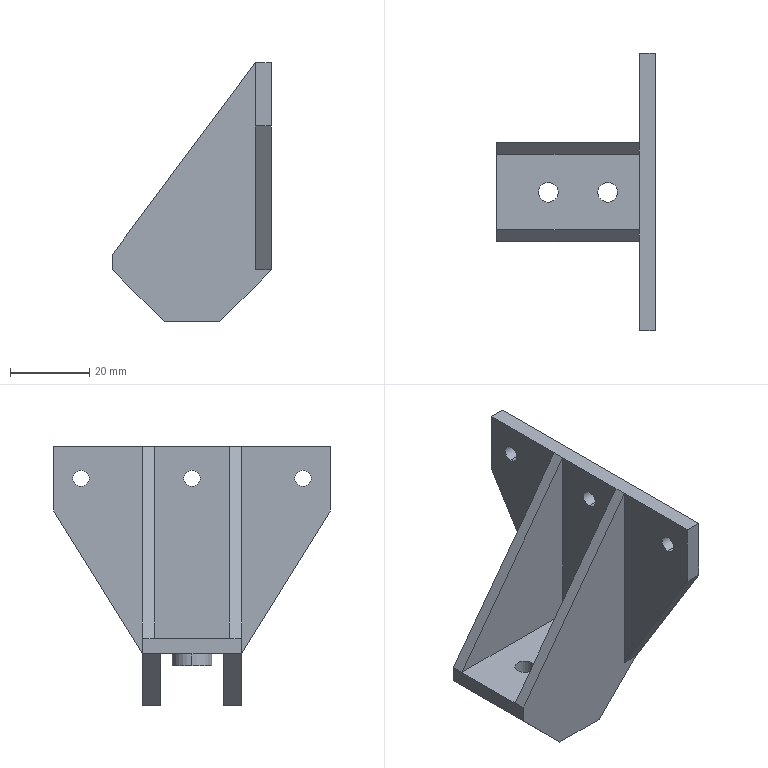Part | STEP file | Weighing fixed frame | 1 solid | 39 faces | box 40 x 70 x 65.291 mm | volume 23281 mm3 | plane 27 | cylinder 12 | commonest cylinder face diameters 4.1 x6 5 x4 10 x2